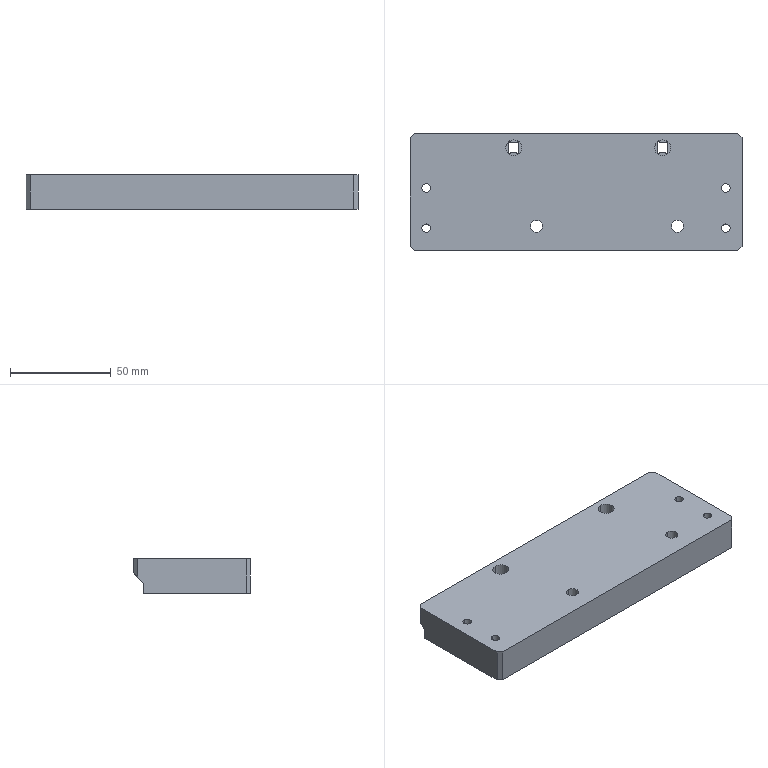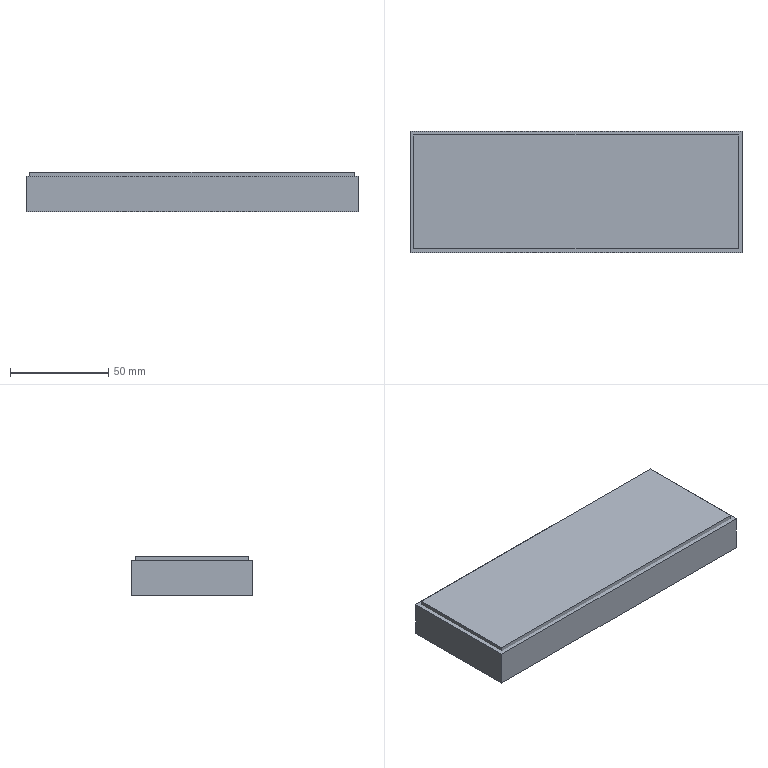CAM job | NX | 3-axis milling, drilling | part box 165 x 58 x 17 mm | stock box 169 x 62 x 20 mm
Tools:
number,name,description,diameter,corner_radius,flute_length,length,flutes
19,D80,Milling Tool-5 Parameters,80.0,0.0,50.0,75.0,2
15,D10,Milling Tool-5 Parameters,10.0,0.0,50.0,75.0,2
1,D6A45,Milling Tool-5 Parameters,6.0,0.0,50.0,75.0,2
14,D10JING,Milling Tool-5 Parameters,10.0,0.0,50.0,75.0,2
12,D6,Milling Tool-5 Parameters,6.0,0.0,50.0,75.0,2
16,D2,Milling Tool-5 Parameters,2.0,0.0,50.0,75.0,2
4,4.2ZT,Drilling Tool,4.2,0.0,35.0,50.0,2
2,2.5ZT,Drilling Tool,2.5,0.0,35.0,50.0,2
11,D4,Milling Tool-5 Parameters,4.0,0.0,50.0,75.0,2
17,D4R0.5,Milling Tool-5 Parameters,4.0,0.5,50.0,75.0,2
Operations:
program,operation,operation_type,tool,method,geometry_group,spindle_rpm,surface_speed,feed_per_tooth,feed_cut,feed_plunge,cut_length_mm,path_length_mm,cut_time_min,machine_time_min
1,FLOOR_WALL,VolumeBased25DMillingOperation,D80,METHOD,A,6500.0,1633.0,0.1154,1500.0,100.0,261.0,315.0,0.174,0.1794
1,ZLEVEL_PROFILE,ZLevelMilling,D10,METHOD,A,9500.0,298.0,0.1579,3000.0,1000.0,8569.522,8643.522,2.888,2.896
1,ZLEVEL_PROFILE_COPY,ZLevelMilling,D10,METHOD,A,9500.0,298.0,0.1579,3000.0,1000.0,1824.509,2351.832,0.6195,0.6722
1,HOLE_MILLING_1,CylinderMilling,D10,METHOD,A,9500.0,298.0,0.0947,1800.0,100.0,198.309,401.309,0.1102,0.1305
1,ZLEVEL_PROFILE_1,ZLevelMilling,D10JING,METHOD,A,9500.0,298.0,0.0789,1500.0,1000.0,481.068,572.068,0.3221,0.3312
1,ZLEVEL_PROFILE_1_COPY,ZLevelMilling,D10JING,METHOD,A,9500.0,298.0,0.0789,1500.0,1000.0,176.022,242.822,0.1187,0.1254
1,ZLEVEL_PROFILE_COPY_1,ZLevelMilling,D6,METHOD,A,9500.0,179.0,0.0789,1500.0,1000.0,532.299,732.629,0.3803,0.4004
1,ZLEVEL_PROFILE_COPY_1_COPY,ZLevelMilling,D2,METHOD,A,9500.0,59.0,0.0526,1000.0,1000.0,1024.905,2174.798,1.025,1.14
1,DRILLING,Operation,D6A45,METHOD,A,9500.0,179.0,0.0132,250.0,0.0,32.0,405.837,0.128,0.1654
1,DRILLING_COPY_COPY,Operation,4.2ZT,METHOD,A,2000.0,21.0,0.0375,150.0,0.0,136.571,537.951,0.9105,0.9506
1,DRILLING_COPY_COPY_COPY,Operation,2.5ZT,METHOD,A,2000.0,21.0,0.0375,150.0,0.0,41.502,220.065,0.2767,0.2945
1,HOLE_MILLING,CylinderMilling,D4,METHOD,A,9500.0,119.0,0.0658,1250.0,100.0,513.002,736.002,0.4104,0.4327
1,ZLEVEL_PROFILE_2,ZLevelMilling,D4R0.5,METHOD,A,9500.0,119.0,0.1579,3000.0,100.0,8953.209,9524.638,2.984,3.042
1,PLANAR_MILL_COPY,PlanarMilling,D6A45,METHOD,A,9500.0,179.0,0.0658,1250.0,100.0,285.931,1123.719,0.2287,0.3125
1,PLANAR_MILL_COPY_COPY,PlanarMilling,D6A45,METHOD,A,9500.0,179.0,0.0658,1250.0,100.0,278.178,337.178,0.2225,0.2284
1,刀补11,CylinderMilling,D4,METHOD,A,9500.0,119.0,0.0658,1250.0,100.0,95.888,318.887,0.0767,0.099
2,FLOOR_WALL_COPY,VolumeBased25DMillingOperation,D80,METHOD,B,6500.0,1633.0,0.1154,1500.0,100.0,771.0,1429.001,0.514,0.5798
2,HOLE_MILLING_1_COPY,CylinderMilling,D4,METHOD,B,9500.0,298.0,0.0947,1800.0,100.0,634.904,845.904,0.3527,0.3738
2,PLANAR_MILL_COPY_COPY_COPY,PlanarMilling,D6A45,METHOD,B,9500.0,179.0,0.0658,1250.0,100.0,588.322,1407.847,0.4707,0.5526